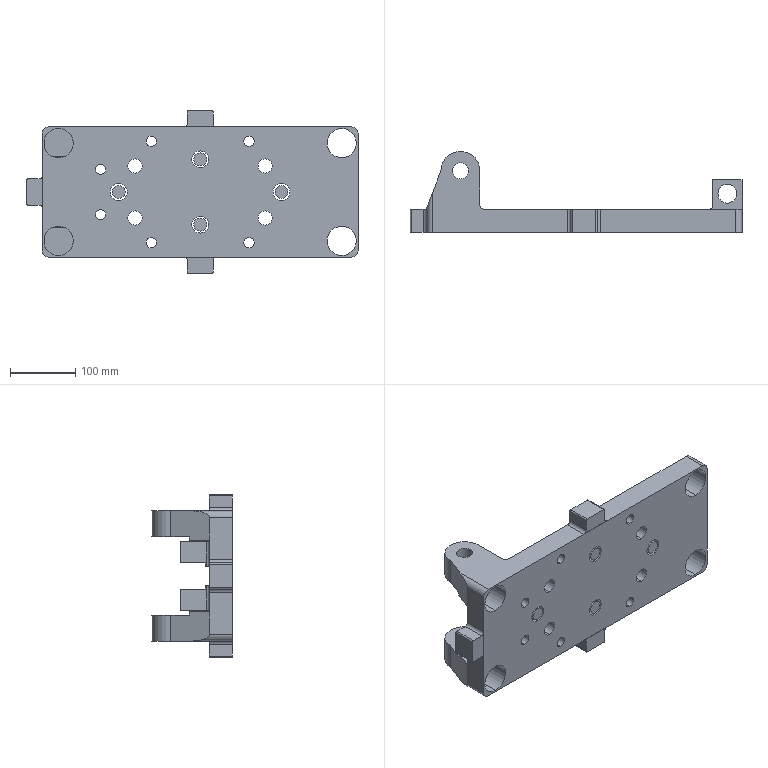Part | SolidWorks | features ICE 6, Extrusion 1, Fillet 1 | 10 solids | 134 faces | box 510.004 x 124.441 x 250 mm | volume 3715115 mm3 | cylinder 74 | plane 60 | commonest cylinder face diameters 16 x12 20 x12 10 x8 22 x8 26 x8 45 x8